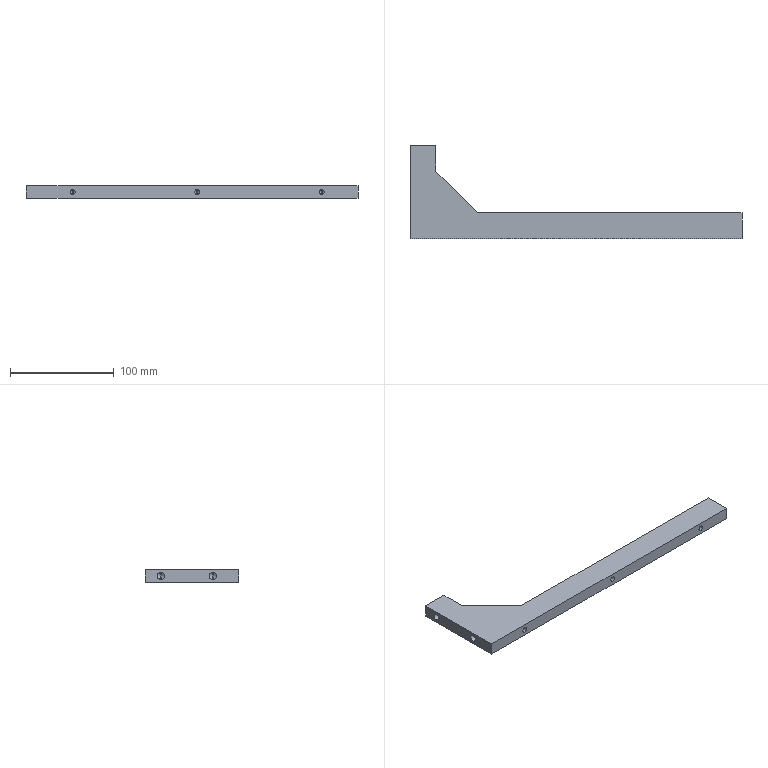Part | SolidWorks | features 3DProfileFeature 2, HoleWzd 2, Extrusion 1 | 1 solid | 29 faces | box 320 x 90 x 12 mm | volume 122776 mm3 | cylinder 10 | cone 10 | plane 9 | commonest cylinder face diameters 5 x6 6.8 x4
STEP:
#1=CARTESIAN_POINT('',(45.,15.,2.5));
#2=VERTEX_POINT('',#1);
#3=CARTESIAN_POINT('',(45.,15.,-2.5));
#4=VERTEX_POINT('',#3);
#5=CARTESIAN_POINT('',(45.,15.,0.));
#6=DIRECTION('',(0.,-1.,0.));
#7=DIRECTION('',(0.,0.,-1.));
#8=AXIS2_PLACEMENT_3D('',#5,#6,#7);
#9=CIRCLE('',#8,2.5);
#10=EDGE_CURVE('',#2,#4,#9,.T.);
#11=ORIENTED_EDGE('',*,*,#10,.F.);
#12=CARTESIAN_POINT('',(45.,0.,2.5));
#13=VERTEX_POINT('',#12);
#14=CARTESIAN_POINT('',(45.,0.,2.5));
#15=DIRECTION('',(0.,-1.,0.));
#16=VECTOR('',#15,1000.);
#17=LINE('',#14,#16);
#18=EDGE_CURVE('',#2,#13,#17,.T.);
#19=ORIENTED_EDGE('',*,*,#18,.T.);
#20=CARTESIAN_POINT('',(45.,0.,-2.5));
#21=VERTEX_POINT('',#20);
#22=CARTESIAN_POINT('',(45.,0.,0.));
#23=DIRECTION('',(0.,-1.,0.));
#24=DIRECTION('',(0.,0.,-1.));
#25=AXIS2_PLACEMENT_3D('',#22,#23,#24);
#26=CIRCLE('',#25,2.5);
#27=EDGE_CURVE('',#13,#21,#26,.T.);
#28=ORIENTED_EDGE('',*,*,#27,.T.);
#29=CARTESIAN_POINT('',(45.,0.,-2.5));
#30=DIRECTION('',(0.,-1.,0.));
#31=VECTOR('',#30,1000.);
#32=LINE('',#29,#31);
#33=EDGE_CURVE('',#4,#21,#32,.T.);
#34=ORIENTED_EDGE('',*,*,#33,.F.);
#35=EDGE_LOOP('',(#11,#19,#28,#34));
#36=FACE_OUTER_BOUND('',#35,.T.);
#37=CARTESIAN_POINT('',(45.,0.,0.));
#38=DIRECTION('',(0.,-1.,0.));
#39=DIRECTION('',(0.,0.,-1.));
#40=AXIS2_PLACEMENT_3D('',#37,#38,#39);
#41=CYLINDRICAL_SURFACE('',#40,2.5);
#42=ADVANCED_FACE('',(#36),#41,.F.);
#43=CARTESIAN_POINT('',(45.,16.502,0.));
#44=VERTEX_POINT('',#43);
#45=CARTESIAN_POINT('',(45.,15.,-2.5));
#46=DIRECTION('',(0.,-0.515,-0.8572));
#47=VECTOR('',#46,1000.);
#48=LINE('',#45,#47);
#49=EDGE_CURVE('',#44,#4,#48,.T.);
#50=ORIENTED_EDGE('',*,*,#49,.F.);
#51=CARTESIAN_POINT('',(45.,15.,2.5));
#52=DIRECTION('',(0.,-0.515,0.8572));
#53=VECTOR('',#52,1000.);
#54=LINE('',#51,#53);
#55=EDGE_CURVE('',#44,#2,#54,.T.);
#56=ORIENTED_EDGE('',*,*,#55,.T.);
#57=ORIENTED_EDGE('',*,*,#10,.T.);
#58=EDGE_LOOP('',(#50,#56,#57));
#59=FACE_OUTER_BOUND('',#58,.T.);
#60=CARTESIAN_POINT('',(45.,15.,0.));
#61=DIRECTION('',(0.,-1.,0.));
#62=DIRECTION('',(0.,0.,-1.));
#63=AXIS2_PLACEMENT_3D('',#60,#61,#62);
#64=CONICAL_SURFACE('',#63,2.5,1.03);
#65=ADVANCED_FACE('',(#59),#64,.F.);
#66=CARTESIAN_POINT('',(165.,15.,2.5));
#67=VERTEX_POINT('',#66);
#68=CARTESIAN_POINT('',(165.,15.,-2.5));
#69=VERTEX_POINT('',#68);
#70=CARTESIAN_POINT('',(165.,15.,0.));
#71=DIRECTION('',(0.,-1.,0.));
#72=DIRECTION('',(0.,0.,-1.));
#73=AXIS2_PLACEMENT_3D('',#70,#71,#72);
#74=CIRCLE('',#73,2.5);
#75=EDGE_CURVE('',#67,#69,#74,.T.);
#76=ORIENTED_EDGE('',*,*,#75,.F.);
#77=CARTESIAN_POINT('',(165.,0.,2.5));
#78=VERTEX_POINT('',#77);
#79=CARTESIAN_POINT('',(165.,0.,2.5));
#80=DIRECTION('',(0.,-1.,0.));
#81=VECTOR('',#80,1000.);
#82=LINE('',#79,#81);
#83=EDGE_CURVE('',#67,#78,#82,.T.);
#84=ORIENTED_EDGE('',*,*,#83,.T.);
#85=CARTESIAN_POINT('',(165.,0.,-2.5));
#86=VERTEX_POINT('',#85);
#87=CARTESIAN_POINT('',(165.,0.,0.));
#88=DIRECTION('',(0.,-1.,0.));
#89=DIRECTION('',(0.,0.,-1.));
#90=AXIS2_PLACEMENT_3D('',#87,#88,#89);
#91=CIRCLE('',#90,2.5);
#92=EDGE_CURVE('',#78,#86,#91,.T.);
#93=ORIENTED_EDGE('',*,*,#92,.T.);
#94=CARTESIAN_POINT('',(165.,0.,-2.5));
#95=DIRECTION('',(0.,-1.,0.));
#96=VECTOR('',#95,1000.);
#97=LINE('',#94,#96);
#98=EDGE_CURVE('',#69,#86,#97,.T.);
#99=ORIENTED_EDGE('',*,*,#98,.F.);
#100=EDGE_LOOP('',(#76,#84,#93,#99));
#101=FACE_OUTER_BOUND('',#100,.T.);
#102=CARTESIAN_POINT('',(165.,0.,0.));
#103=DIRECTION('',(0.,-1.,0.));
#104=DIRECTION('',(0.,0.,-1.));
#105=AXIS2_PLACEMENT_3D('',#102,#103,#104);
#106=CYLINDRICAL_SURFACE('',#105,2.5);
#107=ADVANCED_FACE('',(#101),#106,.F.);
#108=CARTESIAN_POINT('',(165.,16.502,0.));
#109=VERTEX_POINT('',#108);
#110=CARTESIAN_POINT('',(165.,15.,-2.5));
#111=DIRECTION('',(0.,-0.515,-0.8572));
#112=VECTOR('',#111,1000.);
#113=LINE('',#110,#112);
#114=EDGE_CURVE('',#109,#69,#113,.T.);
#115=ORIENTED_EDGE('',*,*,#114,.F.);
#116=CARTESIAN_POINT('',(165.,15.,2.5));
#117=DIRECTION('',(0.,-0.515,0.8572));
#118=VECTOR('',#117,1000.);
#119=LINE('',#116,#118);
#120=EDGE_CURVE('',#109,#67,#119,.T.);
#121=ORIENTED_EDGE('',*,*,#120,.T.);
#122=ORIENTED_EDGE('',*,*,#75,.T.);
#123=EDGE_LOOP('',(#115,#121,#122));
#124=FACE_OUTER_BOUND('',#123,.T.);
#125=CARTESIAN_POINT('',(165.,15.,0.));
#126=DIRECTION('',(0.,-1.,0.));
#127=DIRECTION('',(0.,0.,-1.));
#128=AXIS2_PLACEMENT_3D('',#125,#126,#127);
#129=CONICAL_SURFACE('',#128,2.5,1.03);
#130=ADVANCED_FACE('',(#124),#129,.F.);
#131=CARTESIAN_POINT('',(285.,15.,2.5));
#132=VERTEX_POINT('',#131);
#133=CARTESIAN_POINT('',(285.,15.,-2.5));
#134=VERTEX_POINT('',#133);
#135=CARTESIAN_POINT('',(285.,15.,0.));
#136=DIRECTION('',(0.,-1.,0.));
#137=DIRECTION('',(0.,0.,-1.));
#138=AXIS2_PLACEMENT_3D('',#135,#136,#137);
#139=CIRCLE('',#138,2.5);
#140=EDGE_CURVE('',#132,#134,#139,.T.);
#141=ORIENTED_EDGE('',*,*,#140,.F.);
#142=CARTESIAN_POINT('',(285.,0.,2.5));
#143=VERTEX_POINT('',#142);
#144=CARTESIAN_POINT('',(285.,0.,2.5));
#145=DIRECTION('',(0.,-1.,0.));
#146=VECTOR('',#145,1000.);
#147=LINE('',#144,#146);
#148=EDGE_CURVE('',#132,#143,#147,.T.);
#149=ORIENTED_EDGE('',*,*,#148,.T.);
#150=CARTESIAN_POINT('',(285.,0.,-2.5));
#151=VERTEX_POINT('',#150);
#152=CARTESIAN_POINT('',(285.,0.,0.));
#153=DIRECTION('',(0.,-1.,0.));
#154=DIRECTION('',(0.,0.,-1.));
#155=AXIS2_PLACEMENT_3D('',#152,#153,#154);
#156=CIRCLE('',#155,2.5);
#157=EDGE_CURVE('',#143,#151,#156,.T.);
#158=ORIENTED_EDGE('',*,*,#157,.T.);
#159=CARTESIAN_POINT('',(285.,0.,-2.5));
#160=DIRECTION('',(0.,-1.,0.));
#161=VECTOR('',#160,1000.);
#162=LINE('',#159,#161);
#163=EDGE_CURVE('',#134,#151,#162,.T.);
#164=ORIENTED_EDGE('',*,*,#163,.F.);
#165=EDGE_LOOP('',(#141,#149,#158,#164));
#166=FACE_OUTER_BOUND('',#165,.T.);
#167=CARTESIAN_POINT('',(285.,0.,0.));
#168=DIRECTION('',(0.,-1.,0.));
#169=DIRECTION('',(0.,0.,-1.));
#170=AXIS2_PLACEMENT_3D('',#167,#168,#169);
#171=CYLINDRICAL_SURFACE('',#170,2.5);
#172=ADVANCED_FACE('',(#166),#171,.F.);
#173=CARTESIAN_POINT('',(285.,16.502,0.));
#174=VERTEX_POINT('',#173);
#175=CARTESIAN_POINT('',(285.,15.,-2.5));
#176=DIRECTION('',(0.,-0.515,-0.8572));
#177=VECTOR('',#176,1000.);
#178=LINE('',#175,#177);
#179=EDGE_CURVE('',#174,#134,#178,.T.);
#180=ORIENTED_EDGE('',*,*,#179,.F.);
#181=CARTESIAN_POINT('',(285.,15.,2.5));
#182=DIRECTION('',(0.,-0.515,0.8572));
#183=VECTOR('',#182,1000.);
#184=LINE('',#181,#183);
#185=EDGE_CURVE('',#174,#132,#184,.T.);
#186=ORIENTED_EDGE('',*,*,#185,.T.);
#187=ORIENTED_EDGE('',*,*,#140,.T.);
#188=EDGE_LOOP('',(#180,#186,#187));
#189=FACE_OUTER_BOUND('',#188,.T.);
#190=CARTESIAN_POINT('',(285.,15.,0.));
#191=DIRECTION('',(0.,-1.,0.));
#192=DIRECTION('',(0.,0.,-1.));
#193=AXIS2_PLACEMENT_3D('',#190,#191,#192);
#194=CONICAL_SURFACE('',#193,2.5,1.03);
#195=ADVANCED_FACE('',(#189),#194,.F.);
#196=CARTESIAN_POINT('',(18.75,75.,-3.4));
#197=VERTEX_POINT('',#196);
#198=CARTESIAN_POINT('',(18.75,75.,3.4));
#199=VERTEX_POINT('',#198);
#200=CARTESIAN_POINT('',(18.75,75.,0.));
#201=DIRECTION('',(-1.,0.,0.));
#202=DIRECTION('',(0.,0.,1.));
#203=AXIS2_PLACEMENT_3D('',#200,#201,#202);
#204=CIRCLE('',#203,3.4);
#205=EDGE_CURVE('',#197,#199,#204,.T.);
#206=ORIENTED_EDGE('',*,*,#205,.F.);
#207=CARTESIAN_POINT('',(0.,75.,-3.4));
#208=VERTEX_POINT('',#207);
#209=CARTESIAN_POINT('',(0.,75.,-3.4));
#210=DIRECTION('',(-1.,0.,0.));
#211=VECTOR('',#210,1000.);
#212=LINE('',#209,#211);
#213=EDGE_CURVE('',#197,#208,#212,.T.);
#214=ORIENTED_EDGE('',*,*,#213,.T.);
#215=CARTESIAN_POINT('',(0.,75.,3.4));
#216=VERTEX_POINT('',#215);
#217=CARTESIAN_POINT('',(0.,75.,0.));
#218=DIRECTION('',(-1.,0.,0.));
#219=DIRECTION('',(0.,0.,1.));
#220=AXIS2_PLACEMENT_3D('',#217,#218,#219);
#221=CIRCLE('',#220,3.4);
#222=EDGE_CURVE('',#208,#216,#221,.T.);
#223=ORIENTED_EDGE('',*,*,#222,.T.);
#224=CARTESIAN_POINT('',(0.,75.,3.4));
#225=DIRECTION('',(-1.,0.,0.));
#226=VECTOR('',#225,1000.);
#227=LINE('',#224,#226);
#228=EDGE_CURVE('',#199,#216,#227,.T.);
#229=ORIENTED_EDGE('',*,*,#228,.F.);
#230=EDGE_LOOP('',(#206,#214,#223,#229));
#231=FACE_OUTER_BOUND('',#230,.T.);
#232=CARTESIAN_POINT('',(0.,75.,0.));
#233=DIRECTION('',(-1.,0.,0.));
#234=DIRECTION('',(0.,0.,1.));
#235=AXIS2_PLACEMENT_3D('',#232,#233,#234);
#236=CYLINDRICAL_SURFACE('',#235,3.4);
#237=ADVANCED_FACE('',(#231),#236,.F.);
#238=CARTESIAN_POINT('',(20.793,75.,0.));
#239=VERTEX_POINT('',#238);
#240=CARTESIAN_POINT('',(18.75,75.,3.4));
#241=DIRECTION('',(-0.515,0.,0.8572));
#242=VECTOR('',#241,1000.);
#243=LINE('',#240,#242);
#244=EDGE_CURVE('',#239,#199,#243,.T.);
#245=ORIENTED_EDGE('',*,*,#244,.F.);
#246=CARTESIAN_POINT('',(18.75,75.,-3.4));
#247=DIRECTION('',(-0.515,0.,-0.8572));
#248=VECTOR('',#247,1000.);
#249=LINE('',#246,#248);
#250=EDGE_CURVE('',#239,#197,#249,.T.);
#251=ORIENTED_EDGE('',*,*,#250,.T.);
#252=ORIENTED_EDGE('',*,*,#205,.T.);
#253=EDGE_LOOP('',(#245,#251,#252));
#254=FACE_OUTER_BOUND('',#253,.T.);
#255=CARTESIAN_POINT('',(18.75,75.,0.));
#256=DIRECTION('',(-1.,0.,0.));
#257=DIRECTION('',(0.,0.,1.));
#258=AXIS2_PLACEMENT_3D('',#255,#256,#257);
#259=CONICAL_SURFACE('',#258,3.4,1.03);
#260=ADVANCED_FACE('',(#254),#259,.F.);
#261=CARTESIAN_POINT('',(18.75,25.,-3.4));
#262=VERTEX_POINT('',#261);
#263=CARTESIAN_POINT('',(18.75,25.,3.4));
#264=VERTEX_POINT('',#263);
#265=CARTESIAN_POINT('',(18.75,25.,0.));
#266=DIRECTION('',(-1.,0.,0.));
#267=DIRECTION('',(0.,0.,1.));
#268=AXIS2_PLACEMENT_3D('',#265,#266,#267);
#269=CIRCLE('',#268,3.4);
#270=EDGE_CURVE('',#262,#264,#269,.T.);
#271=ORIENTED_EDGE('',*,*,#270,.F.);
#272=CARTESIAN_POINT('',(0.,25.,-3.4));
#273=VERTEX_POINT('',#272);
#274=CARTESIAN_POINT('',(0.,25.,-3.4));
#275=DIRECTION('',(-1.,0.,0.));
#276=VECTOR('',#275,1000.);
#277=LINE('',#274,#276);
#278=EDGE_CURVE('',#262,#273,#277,.T.);
#279=ORIENTED_EDGE('',*,*,#278,.T.);
#280=CARTESIAN_POINT('',(0.,25.,3.4));
#281=VERTEX_POINT('',#280);
#282=CARTESIAN_POINT('',(0.,25.,0.));
#283=DIRECTION('',(-1.,0.,0.));
#284=DIRECTION('',(0.,0.,1.));
#285=AXIS2_PLACEMENT_3D('',#282,#283,#284);
#286=CIRCLE('',#285,3.4);
#287=EDGE_CURVE('',#273,#281,#286,.T.);
#288=ORIENTED_EDGE('',*,*,#287,.T.);
#289=CARTESIAN_POINT('',(0.,25.,3.4));
#290=DIRECTION('',(-1.,0.,0.));
#291=VECTOR('',#290,1000.);
#292=LINE('',#289,#291);
#293=EDGE_CURVE('',#264,#281,#292,.T.);
#294=ORIENTED_EDGE('',*,*,#293,.F.);
#295=EDGE_LOOP('',(#271,#279,#288,#294));
#296=FACE_OUTER_BOUND('',#295,.T.);
#297=CARTESIAN_POINT('',(0.,25.,0.));
#298=DIRECTION('',(-1.,0.,0.));
#299=DIRECTION('',(0.,0.,1.));
#300=AXIS2_PLACEMENT_3D('',#297,#298,#299);
#301=CYLINDRICAL_SURFACE('',#300,3.4);
#302=ADVANCED_FACE('',(#296),#301,.F.);
#303=CARTESIAN_POINT('',(20.793,25.,0.));
#304=VERTEX_POINT('',#303);
#305=CARTESIAN_POINT('',(18.75,25.,3.4));
#306=DIRECTION('',(-0.515,0.,0.8572));
#307=VECTOR('',#306,1000.);
#308=LINE('',#305,#307);
#309=EDGE_CURVE('',#304,#264,#308,.T.);
#310=ORIENTED_EDGE('',*,*,#309,.F.);
#311=CARTESIAN_POINT('',(18.75,25.,-3.4));
#312=DIRECTION('',(-0.515,0.,-0.8572));
#313=VECTOR('',#312,1000.);
#314=LINE('',#311,#313);
#315=EDGE_CURVE('',#304,#262,#314,.T.);
#316=ORIENTED_EDGE('',*,*,#315,.T.);
#317=ORIENTED_EDGE('',*,*,#270,.T.);
#318=EDGE_LOOP('',(#310,#316,#317));
#319=FACE_OUTER_BOUND('',#318,.T.);
#320=CARTESIAN_POINT('',(18.75,25.,0.));
#321=DIRECTION('',(-1.,0.,0.));
#322=DIRECTION('',(0.,0.,1.));
#323=AXIS2_PLACEMENT_3D('',#320,#321,#322);
#324=CONICAL_SURFACE('',#323,3.4,1.03);
#325=ADVANCED_FACE('',(#319),#324,.F.);
#326=CARTESIAN_POINT('',(45.,0.,0.));
#327=DIRECTION('',(0.,-1.,0.));
#328=DIRECTION('',(0.,0.,-1.));
#329=AXIS2_PLACEMENT_3D('',#326,#327,#328);
#330=CIRCLE('',#329,2.5);
#331=EDGE_CURVE('',#21,#13,#330,.T.);
#332=ORIENTED_EDGE('',*,*,#331,.F.);
#333=ORIENTED_EDGE('',*,*,#27,.F.);
#334=EDGE_LOOP('',(#332,#333));
#335=FACE_BOUND('',#334,.T.);
#336=CARTESIAN_POINT('',(165.,0.,0.));
#337=DIRECTION('',(0.,-1.,0.));
#338=DIRECTION('',(0.,0.,-1.));
#339=AXIS2_PLACEMENT_3D('',#336,#337,#338);
#340=CIRCLE('',#339,2.5);
#341=EDGE_CURVE('',#86,#78,#340,.T.);
#342=ORIENTED_EDGE('',*,*,#341,.F.);
#343=ORIENTED_EDGE('',*,*,#92,.F.);
#344=EDGE_LOOP('',(#342,#343));
#345=FACE_BOUND('',#344,.T.);
#346=CARTESIAN_POINT('',(285.,0.,0.));
#347=DIRECTION('',(0.,-1.,0.));
#348=DIRECTION('',(0.,0.,-1.));
#349=AXIS2_PLACEMENT_3D('',#346,#347,#348);
#350=CIRCLE('',#349,2.5);
#351=EDGE_CURVE('',#151,#143,#350,.T.);
#352=ORIENTED_EDGE('',*,*,#351,.F.);
#353=ORIENTED_EDGE('',*,*,#157,.F.);
#354=EDGE_LOOP('',(#352,#353));
#355=FACE_BOUND('',#354,.T.);
#356=CARTESIAN_POINT('',(0.,0.,-6.));
#357=VERTEX_POINT('',#356);
#358=CARTESIAN_POINT('',(320.,0.,-6.));
#359=VERTEX_POINT('',#358);
#360=CARTESIAN_POINT('',(320.,0.,-6.));
#361=DIRECTION('',(1.,0.,0.));
#362=VECTOR('',#361,1000.);
#363=LINE('',#360,#362);
#364=EDGE_CURVE('',#357,#359,#363,.T.);
#365=ORIENTED_EDGE('',*,*,#364,.T.);
#366=CARTESIAN_POINT('',(320.,0.,6.));
#367=VERTEX_POINT('',#366);
#368=CARTESIAN_POINT('',(320.,0.,6.));
#369=DIRECTION('',(0.,0.,-1.));
#370=VECTOR('',#369,1000.);
#371=LINE('',#368,#370);
#372=EDGE_CURVE('',#367,#359,#371,.T.);
#373=ORIENTED_EDGE('',*,*,#372,.F.);
#374=CARTESIAN_POINT('',(0.,0.,6.));
#375=VERTEX_POINT('',#374);
#376=CARTESIAN_POINT('',(320.,0.,6.));
#377=DIRECTION('',(1.,0.,0.));
#378=VECTOR('',#377,1000.);
#379=LINE('',#376,#378);
#380=EDGE_CURVE('',#375,#367,#379,.T.);
#381=ORIENTED_EDGE('',*,*,#380,.F.);
#382=CARTESIAN_POINT('',(0.,0.,6.));
#383=DIRECTION('',(0.,0.,-1.));
#384=VECTOR('',#383,1000.);
#385=LINE('',#382,#384);
#386=EDGE_CURVE('',#375,#357,#385,.T.);
#387=ORIENTED_EDGE('',*,*,#386,.T.);
#388=EDGE_LOOP('',(#365,#373,#381,#387));
#389=FACE_OUTER_BOUND('',#388,.T.);
#390=CARTESIAN_POINT('',(320.,0.,6.));
#391=DIRECTION('',(0.,1.,0.));
#392=DIRECTION('',(-1.,0.,0.));
#393=AXIS2_PLACEMENT_3D('',#390,#391,#392);
#394=PLANE('',#393);
#395=ADVANCED_FACE('',(#335,#345,#355,#389),#394,.F.);
#396=CARTESIAN_POINT('',(320.,25.,-6.));
#397=VERTEX_POINT('',#396);
#398=CARTESIAN_POINT('',(320.,25.,-6.));
#399=DIRECTION('',(0.,1.,0.));
#400=VECTOR('',#399,1000.);
#401=LINE('',#398,#400);
#402=EDGE_CURVE('',#359,#397,#401,.T.);
#403=ORIENTED_EDGE('',*,*,#402,.T.);
#404=CARTESIAN_POINT('',(320.,25.,6.));
#405=VERTEX_POINT('',#404);
#406=CARTESIAN_POINT('',(320.,25.,6.));
#407=DIRECTION('',(0.,0.,-1.));
#408=VECTOR('',#407,1000.);
#409=LINE('',#406,#408);
#410=EDGE_CURVE('',#405,#397,#409,.T.);
#411=ORIENTED_EDGE('',*,*,#410,.F.);
#412=CARTESIAN_POINT('',(320.,25.,6.));
#413=DIRECTION('',(0.,1.,0.));
#414=VECTOR('',#413,1000.);
#415=LINE('',#412,#414);
#416=EDGE_CURVE('',#367,#405,#415,.T.);
#417=ORIENTED_EDGE('',*,*,#416,.F.);
#418=ORIENTED_EDGE('',*,*,#372,.T.);
#419=EDGE_LOOP('',(#403,#411,#417,#418));
#420=FACE_OUTER_BOUND('',#419,.T.);
#421=CARTESIAN_POINT('',(320.,25.,6.));
#422=DIRECTION('',(-1.,0.,0.));
#423=DIRECTION('',(0.,0.,1.));
#424=AXIS2_PLACEMENT_3D('',#421,#422,#423);
#425=PLANE('',#424);
#426=ADVANCED_FACE('',(#420),#425,.F.);
#427=CARTESIAN_POINT('',(65.,25.,-6.));
#428=VERTEX_POINT('',#427);
#429=CARTESIAN_POINT('',(65.,25.,-6.));
#430=DIRECTION('',(-1.,0.,0.));
#431=VECTOR('',#430,1000.);
#432=LINE('',#429,#431);
#433=EDGE_CURVE('',#397,#428,#432,.T.);
#434=ORIENTED_EDGE('',*,*,#433,.T.);
#435=CARTESIAN_POINT('',(65.,25.,6.));
#436=VERTEX_POINT('',#435);
#437=CARTESIAN_POINT('',(65.,25.,6.));
#438=DIRECTION('',(0.,0.,-1.));
#439=VECTOR('',#438,1000.);
#440=LINE('',#437,#439);
#441=EDGE_CURVE('',#436,#428,#440,.T.);
#442=ORIENTED_EDGE('',*,*,#441,.F.);
#443=CARTESIAN_POINT('',(65.,25.,6.));
#444=DIRECTION('',(-1.,0.,0.));
#445=VECTOR('',#444,1000.);
#446=LINE('',#443,#445);
#447=EDGE_CURVE('',#405,#436,#446,.T.);
#448=ORIENTED_EDGE('',*,*,#447,.F.);
#449=ORIENTED_EDGE('',*,*,#410,.T.);
#450=EDGE_LOOP('',(#434,#442,#448,#449));
#451=FACE_OUTER_BOUND('',#450,.T.);
#452=CARTESIAN_POINT('',(65.,25.,6.));
#453=DIRECTION('',(0.,-1.,0.));
#454=DIRECTION('',(1.,0.,0.));
#455=AXIS2_PLACEMENT_3D('',#452,#453,#454);
#456=PLANE('',#455);
#457=ADVANCED_FACE('',(#451),#456,.F.);
#458=CARTESIAN_POINT('',(25.,65.,-6.));
#459=VERTEX_POINT('',#458);
#460=CARTESIAN_POINT('',(25.,65.,-6.));
#461=DIRECTION('',(-0.7071,0.7071,0.));
#462=VECTOR('',#461,1000.);
#463=LINE('',#460,#462);
#464=EDGE_CURVE('',#428,#459,#463,.T.);
#465=ORIENTED_EDGE('',*,*,#464,.T.);
#466=CARTESIAN_POINT('',(25.,65.,6.));
#467=VERTEX_POINT('',#466);
#468=CARTESIAN_POINT('',(25.,65.,6.));
#469=DIRECTION('',(0.,0.,-1.));
#470=VECTOR('',#469,1000.);
#471=LINE('',#468,#470);
#472=EDGE_CURVE('',#467,#459,#471,.T.);
#473=ORIENTED_EDGE('',*,*,#472,.F.);
#474=CARTESIAN_POINT('',(25.,65.,6.));
#475=DIRECTION('',(-0.7071,0.7071,0.));
#476=VECTOR('',#475,1000.);
#477=LINE('',#474,#476);
#478=EDGE_CURVE('',#436,#467,#477,.T.);
#479=ORIENTED_EDGE('',*,*,#478,.F.);
#480=ORIENTED_EDGE('',*,*,#441,.T.);
#481=EDGE_LOOP('',(#465,#473,#479,#480));
#482=FACE_OUTER_BOUND('',#481,.T.);
#483=CARTESIAN_POINT('',(25.,65.,6.));
#484=DIRECTION('',(-0.7071,-0.7071,0.));
#485=DIRECTION('',(0.7071,-0.7071,0.));
#486=AXIS2_PLACEMENT_3D('',#483,#484,#485);
#487=PLANE('',#486);
#488=ADVANCED_FACE('',(#482),#487,.F.);
#489=CARTESIAN_POINT('',(25.,90.,-6.));
#490=VERTEX_POINT('',#489);
#491=CARTESIAN_POINT('',(25.,90.,-6.));
#492=DIRECTION('',(0.,1.,0.));
#493=VECTOR('',#492,1000.);
#494=LINE('',#491,#493);
#495=EDGE_CURVE('',#459,#490,#494,.T.);
#496=ORIENTED_EDGE('',*,*,#495,.T.);
#497=CARTESIAN_POINT('',(25.,90.,6.));
#498=VERTEX_POINT('',#497);
#499=CARTESIAN_POINT('',(25.,90.,6.));
#500=DIRECTION('',(0.,0.,-1.));
#501=VECTOR('',#500,1000.);
#502=LINE('',#499,#501);
#503=EDGE_CURVE('',#498,#490,#502,.T.);
#504=ORIENTED_EDGE('',*,*,#503,.F.);
#505=CARTESIAN_POINT('',(25.,90.,6.));
#506=DIRECTION('',(0.,1.,0.));
#507=VECTOR('',#506,1000.);
#508=LINE('',#505,#507);
#509=EDGE_CURVE('',#467,#498,#508,.T.);
#510=ORIENTED_EDGE('',*,*,#509,.F.);
#511=ORIENTED_EDGE('',*,*,#472,.T.);
#512=EDGE_LOOP('',(#496,#504,#510,#511));
#513=FACE_OUTER_BOUND('',#512,.T.);
#514=CARTESIAN_POINT('',(25.,90.,6.));
#515=DIRECTION('',(-1.,0.,0.));
#516=DIRECTION('',(0.,-1.,0.));
#517=AXIS2_PLACEMENT_3D('',#514,#515,#516);
#518=PLANE('',#517);
#519=ADVANCED_FACE('',(#513),#518,.F.);
#520=CARTESIAN_POINT('',(0.,90.,-6.));
#521=VERTEX_POINT('',#520);
#522=CARTESIAN_POINT('',(0.,90.,-6.));
#523=DIRECTION('',(-1.,0.,0.));
#524=VECTOR('',#523,1000.);
#525=LINE('',#522,#524);
#526=EDGE_CURVE('',#490,#521,#525,.T.);
#527=ORIENTED_EDGE('',*,*,#526,.T.);
#528=CARTESIAN_POINT('',(0.,90.,6.));
#529=VERTEX_POINT('',#528);
#530=CARTESIAN_POINT('',(0.,90.,6.));
#531=DIRECTION('',(0.,0.,-1.));
#532=VECTOR('',#531,1000.);
#533=LINE('',#530,#532);
#534=EDGE_CURVE('',#529,#521,#533,.T.);
#535=ORIENTED_EDGE('',*,*,#534,.F.);
#536=CARTESIAN_POINT('',(0.,90.,6.));
#537=DIRECTION('',(-1.,0.,0.));
#538=VECTOR('',#537,1000.);
#539=LINE('',#536,#538);
#540=EDGE_CURVE('',#498,#529,#539,.T.);
#541=ORIENTED_EDGE('',*,*,#540,.F.);
#542=ORIENTED_EDGE('',*,*,#503,.T.);
#543=EDGE_LOOP('',(#527,#535,#541,#542));
#544=FACE_OUTER_BOUND('',#543,.T.);
#545=CARTESIAN_POINT('',(0.,90.,6.));
#546=DIRECTION('',(0.,-1.,0.));
#547=DIRECTION('',(0.,0.,-1.));
#548=AXIS2_PLACEMENT_3D('',#545,#546,#547);
#549=PLANE('',#548);
#550=ADVANCED_FACE('',(#544),#549,.F.);
#551=CARTESIAN_POINT('',(0.,75.,0.));
#552=DIRECTION('',(-1.,0.,0.));
#553=DIRECTION('',(0.,0.,1.));
#554=AXIS2_PLACEMENT_3D('',#551,#552,#553);
#555=CIRCLE('',#554,3.4);
#556=EDGE_CURVE('',#216,#208,#555,.T.);
#557=ORIENTED_EDGE('',*,*,#556,.F.);
#558=ORIENTED_EDGE('',*,*,#222,.F.);
#559=EDGE_LOOP('',(#557,#558));
#560=FACE_BOUND('',#559,.T.);
#561=CARTESIAN_POINT('',(0.,25.,0.));
#562=DIRECTION('',(-1.,0.,0.));
#563=DIRECTION('',(0.,0.,1.));
#564=AXIS2_PLACEMENT_3D('',#561,#562,#563);
#565=CIRCLE('',#564,3.4);
#566=EDGE_CURVE('',#281,#273,#565,.T.);
#567=ORIENTED_EDGE('',*,*,#566,.F.);
#568=ORIENTED_EDGE('',*,*,#287,.F.);
#569=EDGE_LOOP('',(#567,#568));
#570=FACE_BOUND('',#569,.T.);
#571=CARTESIAN_POINT('',(0.,0.,-6.));
#572=DIRECTION('',(0.,-1.,0.));
#573=VECTOR('',#572,1000.);
#574=LINE('',#571,#573);
#575=EDGE_CURVE('',#521,#357,#574,.T.);
#576=ORIENTED_EDGE('',*,*,#575,.T.);
#577=ORIENTED_EDGE('',*,*,#386,.F.);
#578=CARTESIAN_POINT('',(0.,0.,6.));
#579=DIRECTION('',(0.,-1.,0.));
#580=VECTOR('',#579,1000.);
#581=LINE('',#578,#580);
#582=EDGE_CURVE('',#529,#375,#581,.T.);
#583=ORIENTED_EDGE('',*,*,#582,.F.);
#584=ORIENTED_EDGE('',*,*,#534,.T.);
#585=EDGE_LOOP('',(#576,#577,#583,#584));
#586=FACE_OUTER_BOUND('',#585,.T.);
#587=CARTESIAN_POINT('',(0.,0.,6.));
#588=DIRECTION('',(1.,0.,0.));
#589=DIRECTION('',(0.,0.,-1.));
#590=AXIS2_PLACEMENT_3D('',#587,#588,#589);
#591=PLANE('',#590);
#592=ADVANCED_FACE('',(#560,#570,#586),#591,.F.);
#593=ORIENTED_EDGE('',*,*,#380,.T.);
#594=ORIENTED_EDGE('',*,*,#416,.T.);
#595=ORIENTED_EDGE('',*,*,#447,.T.);
#596=ORIENTED_EDGE('',*,*,#478,.T.);
#597=ORIENTED_EDGE('',*,*,#509,.T.);
#598=ORIENTED_EDGE('',*,*,#540,.T.);
#599=ORIENTED_EDGE('',*,*,#582,.T.);
#600=EDGE_LOOP('',(#593,#594,#595,#596,#597,#598,#599));
#601=FACE_OUTER_BOUND('',#600,.T.);
#602=CARTESIAN_POINT('',(0.,0.,6.));
#603=DIRECTION('',(0.,0.,-1.));
#604=DIRECTION('',(-1.,0.,0.));
#605=AXIS2_PLACEMENT_3D('',#602,#603,#604);
#606=PLANE('',#605);
#607=ADVANCED_FACE('',(#601),#606,.F.);
#608=ORIENTED_EDGE('',*,*,#364,.F.);
#609=ORIENTED_EDGE('',*,*,#575,.F.);
#610=ORIENTED_EDGE('',*,*,#526,.F.);
#611=ORIENTED_EDGE('',*,*,#495,.F.);
#612=ORIENTED_EDGE('',*,*,#464,.F.);
#613=ORIENTED_EDGE('',*,*,#433,.F.);
#614=ORIENTED_EDGE('',*,*,#402,.F.);
#615=EDGE_LOOP('',(#608,#609,#610,#611,#612,#613,#614));
#616=FACE_OUTER_BOUND('',#615,.T.);
#617=CARTESIAN_POINT('',(0.,0.,-6.));
#618=DIRECTION('',(0.,0.,-1.));
#619=DIRECTION('',(-1.,0.,0.));
#620=AXIS2_PLACEMENT_3D('',#617,#618,#619);
#621=PLANE('',#620);
#622=ADVANCED_FACE('',(#616),#621,.T.);
#623=ORIENTED_EDGE('',*,*,#315,.F.);
#624=ORIENTED_EDGE('',*,*,#309,.T.);
#625=CARTESIAN_POINT('',(18.75,25.,0.));
#626=DIRECTION('',(-1.,0.,0.));
#627=DIRECTION('',(0.,0.,1.));
#628=AXIS2_PLACEMENT_3D('',#625,#626,#627);
#629=CIRCLE('',#628,3.4);
#630=EDGE_CURVE('',#264,#262,#629,.T.);
#631=ORIENTED_EDGE('',*,*,#630,.T.);
#632=EDGE_LOOP('',(#623,#624,#631));
#633=FACE_OUTER_BOUND('',#632,.T.);
#634=CARTESIAN_POINT('',(18.75,25.,0.));
#635=DIRECTION('',(-1.,0.,0.));
#636=DIRECTION('',(0.,0.,1.));
#637=AXIS2_PLACEMENT_3D('',#634,#635,#636);
#638=CONICAL_SURFACE('',#637,3.4,1.03);
#639=ADVANCED_FACE('',(#633),#638,.F.);
#640=ORIENTED_EDGE('',*,*,#278,.F.);
#641=ORIENTED_EDGE('',*,*,#630,.F.);
#642=ORIENTED_EDGE('',*,*,#293,.T.);
#643=ORIENTED_EDGE('',*,*,#566,.T.);
#644=EDGE_LOOP('',(#640,#641,#642,#643));
#645=FACE_OUTER_BOUND('',#644,.T.);
#646=CARTESIAN_POINT('',(0.,25.,0.));
#647=DIRECTION('',(-1.,0.,0.));
#648=DIRECTION('',(0.,0.,1.));
#649=AXIS2_PLACEMENT_3D('',#646,#647,#648);
#650=CYLINDRICAL_SURFACE('',#649,3.4);
#651=ADVANCED_FACE('',(#645),#650,.F.);
#652=ORIENTED_EDGE('',*,*,#250,.F.);
#653=ORIENTED_EDGE('',*,*,#244,.T.);
#654=CARTESIAN_POINT('',(18.75,75.,0.));
#655=DIRECTION('',(-1.,0.,0.));
#656=DIRECTION('',(0.,0.,1.));
#657=AXIS2_PLACEMENT_3D('',#654,#655,#656);
#658=CIRCLE('',#657,3.4);
#659=EDGE_CURVE('',#199,#197,#658,.T.);
#660=ORIENTED_EDGE('',*,*,#659,.T.);
#661=EDGE_LOOP('',(#652,#653,#660));
#662=FACE_OUTER_BOUND('',#661,.T.);
#663=CARTESIAN_POINT('',(18.75,75.,0.));
#664=DIRECTION('',(-1.,0.,0.));
#665=DIRECTION('',(0.,0.,1.));
#666=AXIS2_PLACEMENT_3D('',#663,#664,#665);
#667=CONICAL_SURFACE('',#666,3.4,1.03);
#668=ADVANCED_FACE('',(#662),#667,.F.);
#669=ORIENTED_EDGE('',*,*,#213,.F.);
#670=ORIENTED_EDGE('',*,*,#659,.F.);
#671=ORIENTED_EDGE('',*,*,#228,.T.);
#672=ORIENTED_EDGE('',*,*,#556,.T.);
#673=EDGE_LOOP('',(#669,#670,#671,#672));
#674=FACE_OUTER_BOUND('',#673,.T.);
#675=CARTESIAN_POINT('',(0.,75.,0.));
#676=DIRECTION('',(-1.,0.,0.));
#677=DIRECTION('',(0.,0.,1.));
#678=AXIS2_PLACEMENT_3D('',#675,#676,#677);
#679=CYLINDRICAL_SURFACE('',#678,3.4);
#680=ADVANCED_FACE('',(#674),#679,.F.);
#681=ORIENTED_EDGE('',*,*,#185,.F.);
#682=ORIENTED_EDGE('',*,*,#179,.T.);
#683=CARTESIAN_POINT('',(285.,15.,0.));
#684=DIRECTION('',(0.,-1.,0.));
#685=DIRECTION('',(0.,0.,-1.));
#686=AXIS2_PLACEMENT_3D('',#683,#684,#685);
#687=CIRCLE('',#686,2.5);
#688=EDGE_CURVE('',#134,#132,#687,.T.);
#689=ORIENTED_EDGE('',*,*,#688,.T.);
#690=EDGE_LOOP('',(#681,#682,#689));
#691=FACE_OUTER_BOUND('',#690,.T.);
#692=CARTESIAN_POINT('',(285.,15.,0.));
#693=DIRECTION('',(0.,-1.,0.));
#694=DIRECTION('',(0.,0.,-1.));
#695=AXIS2_PLACEMENT_3D('',#692,#693,#694);
#696=CONICAL_SURFACE('',#695,2.5,1.03);
#697=ADVANCED_FACE('',(#691),#696,.F.);
#698=ORIENTED_EDGE('',*,*,#148,.F.);
#699=ORIENTED_EDGE('',*,*,#688,.F.);
#700=ORIENTED_EDGE('',*,*,#163,.T.);
#701=ORIENTED_EDGE('',*,*,#351,.T.);
#702=EDGE_LOOP('',(#698,#699,#700,#701));
#703=FACE_OUTER_BOUND('',#702,.T.);
#704=CARTESIAN_POINT('',(285.,0.,0.));
#705=DIRECTION('',(0.,-1.,0.));
#706=DIRECTION('',(0.,0.,-1.));
#707=AXIS2_PLACEMENT_3D('',#704,#705,#706);
#708=CYLINDRICAL_SURFACE('',#707,2.5);
#709=ADVANCED_FACE('',(#703),#708,.F.);
#710=ORIENTED_EDGE('',*,*,#120,.F.);
#711=ORIENTED_EDGE('',*,*,#114,.T.);
#712=CARTESIAN_POINT('',(165.,15.,0.));
#713=DIRECTION('',(0.,-1.,0.));
#714=DIRECTION('',(0.,0.,-1.));
#715=AXIS2_PLACEMENT_3D('',#712,#713,#714);
#716=CIRCLE('',#715,2.5);
#717=EDGE_CURVE('',#69,#67,#716,.T.);
#718=ORIENTED_EDGE('',*,*,#717,.T.);
#719=EDGE_LOOP('',(#710,#711,#718));
#720=FACE_OUTER_BOUND('',#719,.T.);
#721=CARTESIAN_POINT('',(165.,15.,0.));
#722=DIRECTION('',(0.,-1.,0.));
#723=DIRECTION('',(0.,0.,-1.));
#724=AXIS2_PLACEMENT_3D('',#721,#722,#723);
#725=CONICAL_SURFACE('',#724,2.5,1.03);
#726=ADVANCED_FACE('',(#720),#725,.F.);
#727=ORIENTED_EDGE('',*,*,#83,.F.);
#728=ORIENTED_EDGE('',*,*,#717,.F.);
#729=ORIENTED_EDGE('',*,*,#98,.T.);
#730=ORIENTED_EDGE('',*,*,#341,.T.);
#731=EDGE_LOOP('',(#727,#728,#729,#730));
#732=FACE_OUTER_BOUND('',#731,.T.);
#733=CARTESIAN_POINT('',(165.,0.,0.));
#734=DIRECTION('',(0.,-1.,0.));
#735=DIRECTION('',(0.,0.,-1.));
#736=AXIS2_PLACEMENT_3D('',#733,#734,#735);
#737=CYLINDRICAL_SURFACE('',#736,2.5);
#738=ADVANCED_FACE('',(#732),#737,.F.);
#739=ORIENTED_EDGE('',*,*,#55,.F.);
#740=ORIENTED_EDGE('',*,*,#49,.T.);
#741=CARTESIAN_POINT('',(45.,15.,0.));
#742=DIRECTION('',(0.,-1.,0.));
#743=DIRECTION('',(0.,0.,-1.));
#744=AXIS2_PLACEMENT_3D('',#741,#742,#743);
#745=CIRCLE('',#744,2.5);
#746=EDGE_CURVE('',#4,#2,#745,.T.);
#747=ORIENTED_EDGE('',*,*,#746,.T.);
#748=EDGE_LOOP('',(#739,#740,#747));
#749=FACE_OUTER_BOUND('',#748,.T.);
#750=CARTESIAN_POINT('',(45.,15.,0.));
#751=DIRECTION('',(0.,-1.,0.));
#752=DIRECTION('',(0.,0.,-1.));
#753=AXIS2_PLACEMENT_3D('',#750,#751,#752);
#754=CONICAL_SURFACE('',#753,2.5,1.03);
#755=ADVANCED_FACE('',(#749),#754,.F.);
#756=ORIENTED_EDGE('',*,*,#18,.F.);
#757=ORIENTED_EDGE('',*,*,#746,.F.);
#758=ORIENTED_EDGE('',*,*,#33,.T.);
#759=ORIENTED_EDGE('',*,*,#331,.T.);
#760=EDGE_LOOP('',(#756,#757,#758,#759));
#761=FACE_OUTER_BOUND('',#760,.T.);
#762=CARTESIAN_POINT('',(45.,0.,0.));
#763=DIRECTION('',(0.,-1.,0.));
#764=DIRECTION('',(0.,0.,-1.));
#765=AXIS2_PLACEMENT_3D('',#762,#763,#764);
#766=CYLINDRICAL_SURFACE('',#765,2.5);
#767=ADVANCED_FACE('',(#761),#766,.F.);
#768=CLOSED_SHELL('',(#42,#65,#107,#130,#172,#195,#237,#260,#302,#325,#395,#426,#457,#488,#519,#550,#592,#607,#622,#639,#651,#668,#680,#697,#709,#726,#738,#755,#767));
#769=MANIFOLD_SOLID_BREP('',#768);
#770=CARTESIAN_POINT('',(0.,0.,0.));
#771=DIRECTION('',(0.,0.,1.));
#772=DIRECTION('',(1.,0.,0.));
#773=AXIS2_PLACEMENT_3D('',#770,#771,#772);
#774=(LENGTH_UNIT()NAMED_UNIT(*)SI_UNIT(.MILLI.,.METRE.));
#775=UNCERTAINTY_MEASURE_WITH_UNIT(LENGTH_MEASURE(0.00001),#774,'','');
#776=(NAMED_UNIT(*)PLANE_ANGLE_UNIT()SI_UNIT($,.RADIAN.));
#777=(NAMED_UNIT(*)SI_UNIT($,.STERADIAN.)SOLID_ANGLE_UNIT());
#778=(GEOMETRIC_REPRESENTATION_CONTEXT(3)GLOBAL_UNCERTAINTY_ASSIGNED_CONTEXT((#775))GLOBAL_UNIT_ASSIGNED_CONTEXT((#774,#776,#777))REPRESENTATION_CONTEXT('',''));
#779=ADVANCED_BREP_SHAPE_REPRESENTATION('',(#769,#773),#778);